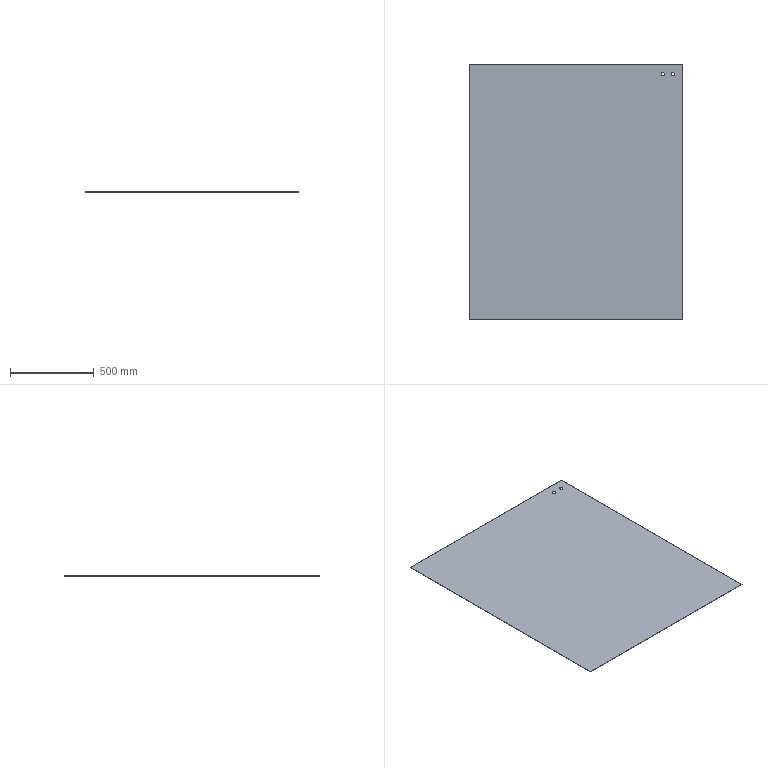Part | STEP file | ASND-0110-E63-HLTP01标准Lower机架-10 | 1 solid | 10 faces | box 1280 x 1530 x 2 mm | volume 3915543 mm3 | plane 6 | cylinder 4 | commonest cylinder face diameters 20 x4
STEP:
#1=CARTESIAN_POINT('',(0.,0.,0.));
#2=DIRECTION('',(0.,0.,1.));
#3=DIRECTION('',(1.,0.,0.));
#4=AXIS2_PLACEMENT_3D('',#1,#2,#3);
#5=CARTESIAN_POINT('',(-110.,-60.,0.));
#6=VERTEX_POINT('',#5);
#7=CARTESIAN_POINT('',(-110.,-60.,2.));
#8=VERTEX_POINT('',#7);
#9=CARTESIAN_POINT('',(-110.,-60.,-8.));
#10=DIRECTION('',(0.,0.,1.));
#11=VECTOR('',#10,1.);
#12=LINE('',#9,#11);
#13=CARTESIAN_POINT('',(-120.,-60.,-8.));
#14=DIRECTION('',(0.,0.,1.));
#15=DIRECTION('',(1.,0.,0.));
#16=AXIS2_PLACEMENT_3D('',#13,#14,#15);
#17=CYLINDRICAL_SURFACE('',#16,10.);
#18=CARTESIAN_POINT('',(6.283,0.));
#19=DIRECTION('',(0.,1.));
#20=VECTOR('',#19,1.);
#21=LINE('',#18,#20);
#22=(GEOMETRIC_REPRESENTATION_CONTEXT(2)PARAMETRIC_REPRESENTATION_CONTEXT()REPRESENTATION_CONTEXT('',''));
#23=DEFINITIONAL_REPRESENTATION('',(#21),#22);
#24=PCURVE('',#17,#23);
#25=CARTESIAN_POINT('',(-120.,-60.,-8.));
#26=DIRECTION('',(0.,0.,1.));
#27=DIRECTION('',(1.,0.,0.));
#28=AXIS2_PLACEMENT_3D('',#25,#26,#27);
#29=CYLINDRICAL_SURFACE('',#28,10.);
#30=CARTESIAN_POINT('',(0.,0.));
#31=DIRECTION('',(0.,1.));
#32=VECTOR('',#31,1.);
#33=LINE('',#30,#32);
#34=(GEOMETRIC_REPRESENTATION_CONTEXT(2)PARAMETRIC_REPRESENTATION_CONTEXT()REPRESENTATION_CONTEXT('',''));
#35=DEFINITIONAL_REPRESENTATION('',(#33),#34);
#36=PCURVE('',#29,#35);
#37=SURFACE_CURVE('',#12,(#24,#36),.PCURVE_S1.);
#38=EDGE_CURVE('',#6,#8,#37,.T.);
#39=ORIENTED_EDGE('',*,*,#38,.T.);
#40=CARTESIAN_POINT('',(-130.,-60.,2.));
#41=VERTEX_POINT('',#40);
#42=CARTESIAN_POINT('',(-120.,-60.,2.));
#43=DIRECTION('',(0.,0.,1.));
#44=DIRECTION('',(1.,0.,0.));
#45=AXIS2_PLACEMENT_3D('',#42,#43,#44);
#46=CIRCLE('',#45,10.);
#47=CARTESIAN_POINT('',(0.,10.));
#48=DIRECTION('',(1.,0.));
#49=VECTOR('',#48,1.);
#50=LINE('',#47,#49);
#51=(GEOMETRIC_REPRESENTATION_CONTEXT(2)PARAMETRIC_REPRESENTATION_CONTEXT()REPRESENTATION_CONTEXT('',''));
#52=DEFINITIONAL_REPRESENTATION('',(#50),#51);
#53=PCURVE('',#17,#52);
#54=CARTESIAN_POINT('',(0.,0.,2.));
#55=DIRECTION('',(0.,0.,1.));
#56=DIRECTION('',(0.7071,0.7071,0.));
#57=AXIS2_PLACEMENT_3D('',#54,#55,#56);
#58=PLANE('',#57);
#59=CARTESIAN_POINT('',(-127.279,42.426));
#60=DIRECTION('',(0.7071,-0.7071));
#61=AXIS2_PLACEMENT_2D('',#59,#60);
#62=CIRCLE('',#61,10.);
#63=(GEOMETRIC_REPRESENTATION_CONTEXT(2)PARAMETRIC_REPRESENTATION_CONTEXT()REPRESENTATION_CONTEXT('',''));
#64=DEFINITIONAL_REPRESENTATION('',(#62),#63);
#65=PCURVE('',#58,#64);
#66=SURFACE_CURVE('',#46,(#53,#65),.PCURVE_S1.);
#67=EDGE_CURVE('',#41,#8,#66,.T.);
#68=ORIENTED_EDGE('',*,*,#67,.F.);
#69=CARTESIAN_POINT('',(-130.,-60.,0.));
#70=VERTEX_POINT('',#69);
#71=CARTESIAN_POINT('',(-130.,-60.,-8.));
#72=DIRECTION('',(0.,0.,1.));
#73=VECTOR('',#72,1.);
#74=LINE('',#71,#73);
#75=CARTESIAN_POINT('',(3.142,0.));
#76=DIRECTION('',(0.,1.));
#77=VECTOR('',#76,1.);
#78=LINE('',#75,#77);
#79=(GEOMETRIC_REPRESENTATION_CONTEXT(2)PARAMETRIC_REPRESENTATION_CONTEXT()REPRESENTATION_CONTEXT('',''));
#80=DEFINITIONAL_REPRESENTATION('',(#78),#79);
#81=PCURVE('',#17,#80);
#82=CARTESIAN_POINT('',(3.142,0.));
#83=DIRECTION('',(0.,1.));
#84=VECTOR('',#83,1.);
#85=LINE('',#82,#84);
#86=(GEOMETRIC_REPRESENTATION_CONTEXT(2)PARAMETRIC_REPRESENTATION_CONTEXT()REPRESENTATION_CONTEXT('',''));
#87=DEFINITIONAL_REPRESENTATION('',(#85),#86);
#88=PCURVE('',#29,#87);
#89=SURFACE_CURVE('',#74,(#81,#88),.PCURVE_S1.);
#90=EDGE_CURVE('',#70,#41,#89,.T.);
#91=ORIENTED_EDGE('',*,*,#90,.F.);
#92=CARTESIAN_POINT('',(-120.,-60.,0.));
#93=DIRECTION('',(0.,0.,1.));
#94=DIRECTION('',(1.,0.,0.));
#95=AXIS2_PLACEMENT_3D('',#92,#93,#94);
#96=CIRCLE('',#95,10.);
#97=CARTESIAN_POINT('',(0.,8.));
#98=DIRECTION('',(1.,0.));
#99=VECTOR('',#98,1.);
#100=LINE('',#97,#99);
#101=(GEOMETRIC_REPRESENTATION_CONTEXT(2)PARAMETRIC_REPRESENTATION_CONTEXT()REPRESENTATION_CONTEXT('',''));
#102=DEFINITIONAL_REPRESENTATION('',(#100),#101);
#103=PCURVE('',#17,#102);
#104=CARTESIAN_POINT('',(0.,0.,0.));
#105=DIRECTION('',(0.,0.,1.));
#106=DIRECTION('',(0.7071,0.7071,0.));
#107=AXIS2_PLACEMENT_3D('',#104,#105,#106);
#108=PLANE('',#107);
#109=CARTESIAN_POINT('',(-127.279,42.426));
#110=DIRECTION('',(0.7071,-0.7071));
#111=AXIS2_PLACEMENT_2D('',#109,#110);
#112=CIRCLE('',#111,10.);
#113=(GEOMETRIC_REPRESENTATION_CONTEXT(2)PARAMETRIC_REPRESENTATION_CONTEXT()REPRESENTATION_CONTEXT('',''));
#114=DEFINITIONAL_REPRESENTATION('',(#112),#113);
#115=PCURVE('',#108,#114);
#116=SURFACE_CURVE('',#96,(#103,#115),.PCURVE_S1.);
#117=EDGE_CURVE('',#70,#6,#116,.T.);
#118=ORIENTED_EDGE('',*,*,#117,.T.);
#119=EDGE_LOOP('',(#39,#68,#91,#118));
#120=FACE_BOUND('',#119,.F.);
#121=ADVANCED_FACE('',(#120),#17,.F.);
#122=CARTESIAN_POINT('',(-170.,-60.,0.));
#123=VERTEX_POINT('',#122);
#124=CARTESIAN_POINT('',(-170.,-60.,2.));
#125=VERTEX_POINT('',#124);
#126=CARTESIAN_POINT('',(-170.,-60.,-8.));
#127=DIRECTION('',(0.,0.,1.));
#128=VECTOR('',#127,1.);
#129=LINE('',#126,#128);
#130=CARTESIAN_POINT('',(-180.,-60.,-8.));
#131=DIRECTION('',(0.,0.,1.));
#132=DIRECTION('',(1.,0.,0.));
#133=AXIS2_PLACEMENT_3D('',#130,#131,#132);
#134=CYLINDRICAL_SURFACE('',#133,10.);
#135=CARTESIAN_POINT('',(6.283,0.));
#136=DIRECTION('',(0.,1.));
#137=VECTOR('',#136,1.);
#138=LINE('',#135,#137);
#139=(GEOMETRIC_REPRESENTATION_CONTEXT(2)PARAMETRIC_REPRESENTATION_CONTEXT()REPRESENTATION_CONTEXT('',''));
#140=DEFINITIONAL_REPRESENTATION('',(#138),#139);
#141=PCURVE('',#134,#140);
#142=CARTESIAN_POINT('',(-180.,-60.,-8.));
#143=DIRECTION('',(0.,0.,1.));
#144=DIRECTION('',(1.,0.,0.));
#145=AXIS2_PLACEMENT_3D('',#142,#143,#144);
#146=CYLINDRICAL_SURFACE('',#145,10.);
#147=CARTESIAN_POINT('',(0.,0.));
#148=DIRECTION('',(0.,1.));
#149=VECTOR('',#148,1.);
#150=LINE('',#147,#149);
#151=(GEOMETRIC_REPRESENTATION_CONTEXT(2)PARAMETRIC_REPRESENTATION_CONTEXT()REPRESENTATION_CONTEXT('',''));
#152=DEFINITIONAL_REPRESENTATION('',(#150),#151);
#153=PCURVE('',#146,#152);
#154=SURFACE_CURVE('',#129,(#141,#153),.PCURVE_S1.);
#155=EDGE_CURVE('',#123,#125,#154,.T.);
#156=ORIENTED_EDGE('',*,*,#155,.T.);
#157=CARTESIAN_POINT('',(-190.,-60.,2.));
#158=VERTEX_POINT('',#157);
#159=CARTESIAN_POINT('',(-180.,-60.,2.));
#160=DIRECTION('',(0.,0.,1.));
#161=DIRECTION('',(1.,0.,0.));
#162=AXIS2_PLACEMENT_3D('',#159,#160,#161);
#163=CIRCLE('',#162,10.);
#164=CARTESIAN_POINT('',(0.,10.));
#165=DIRECTION('',(1.,0.));
#166=VECTOR('',#165,1.);
#167=LINE('',#164,#166);
#168=(GEOMETRIC_REPRESENTATION_CONTEXT(2)PARAMETRIC_REPRESENTATION_CONTEXT()REPRESENTATION_CONTEXT('',''));
#169=DEFINITIONAL_REPRESENTATION('',(#167),#168);
#170=PCURVE('',#134,#169);
#171=CARTESIAN_POINT('',(-169.706,84.853));
#172=DIRECTION('',(0.7071,-0.7071));
#173=AXIS2_PLACEMENT_2D('',#171,#172);
#174=CIRCLE('',#173,10.);
#175=(GEOMETRIC_REPRESENTATION_CONTEXT(2)PARAMETRIC_REPRESENTATION_CONTEXT()REPRESENTATION_CONTEXT('',''));
#176=DEFINITIONAL_REPRESENTATION('',(#174),#175);
#177=PCURVE('',#58,#176);
#178=SURFACE_CURVE('',#163,(#170,#177),.PCURVE_S1.);
#179=EDGE_CURVE('',#158,#125,#178,.T.);
#180=ORIENTED_EDGE('',*,*,#179,.F.);
#181=CARTESIAN_POINT('',(-190.,-60.,0.));
#182=VERTEX_POINT('',#181);
#183=CARTESIAN_POINT('',(-190.,-60.,-8.));
#184=DIRECTION('',(0.,0.,1.));
#185=VECTOR('',#184,1.);
#186=LINE('',#183,#185);
#187=CARTESIAN_POINT('',(3.142,0.));
#188=DIRECTION('',(0.,1.));
#189=VECTOR('',#188,1.);
#190=LINE('',#187,#189);
#191=(GEOMETRIC_REPRESENTATION_CONTEXT(2)PARAMETRIC_REPRESENTATION_CONTEXT()REPRESENTATION_CONTEXT('',''));
#192=DEFINITIONAL_REPRESENTATION('',(#190),#191);
#193=PCURVE('',#134,#192);
#194=CARTESIAN_POINT('',(3.142,0.));
#195=DIRECTION('',(0.,1.));
#196=VECTOR('',#195,1.);
#197=LINE('',#194,#196);
#198=(GEOMETRIC_REPRESENTATION_CONTEXT(2)PARAMETRIC_REPRESENTATION_CONTEXT()REPRESENTATION_CONTEXT('',''));
#199=DEFINITIONAL_REPRESENTATION('',(#197),#198);
#200=PCURVE('',#146,#199);
#201=SURFACE_CURVE('',#186,(#193,#200),.PCURVE_S1.);
#202=EDGE_CURVE('',#182,#158,#201,.T.);
#203=ORIENTED_EDGE('',*,*,#202,.F.);
#204=CARTESIAN_POINT('',(-180.,-60.,0.));
#205=DIRECTION('',(0.,0.,1.));
#206=DIRECTION('',(1.,0.,0.));
#207=AXIS2_PLACEMENT_3D('',#204,#205,#206);
#208=CIRCLE('',#207,10.);
#209=CARTESIAN_POINT('',(0.,8.));
#210=DIRECTION('',(1.,0.));
#211=VECTOR('',#210,1.);
#212=LINE('',#209,#211);
#213=(GEOMETRIC_REPRESENTATION_CONTEXT(2)PARAMETRIC_REPRESENTATION_CONTEXT()REPRESENTATION_CONTEXT('',''));
#214=DEFINITIONAL_REPRESENTATION('',(#212),#213);
#215=PCURVE('',#134,#214);
#216=CARTESIAN_POINT('',(-169.706,84.853));
#217=DIRECTION('',(0.7071,-0.7071));
#218=AXIS2_PLACEMENT_2D('',#216,#217);
#219=CIRCLE('',#218,10.);
#220=(GEOMETRIC_REPRESENTATION_CONTEXT(2)PARAMETRIC_REPRESENTATION_CONTEXT()REPRESENTATION_CONTEXT('',''));
#221=DEFINITIONAL_REPRESENTATION('',(#219),#220);
#222=PCURVE('',#108,#221);
#223=SURFACE_CURVE('',#208,(#215,#222),.PCURVE_S1.);
#224=EDGE_CURVE('',#182,#123,#223,.T.);
#225=ORIENTED_EDGE('',*,*,#224,.T.);
#226=EDGE_LOOP('',(#156,#180,#203,#225));
#227=FACE_BOUND('',#226,.F.);
#228=ADVANCED_FACE('',(#227),#134,.F.);
#229=CARTESIAN_POINT('',(-1340.,0.,0.));
#230=VERTEX_POINT('',#229);
#231=CARTESIAN_POINT('',(-1340.,-1530.,0.));
#232=VERTEX_POINT('',#231);
#233=CARTESIAN_POINT('',(-1340.,0.,0.));
#234=DIRECTION('',(0.,-1.,0.));
#235=VECTOR('',#234,1.);
#236=LINE('',#233,#235);
#237=CARTESIAN_POINT('',(-1340.,0.,2.));
#238=DIRECTION('',(1.,0.,0.));
#239=DIRECTION('',(0.,0.7071,0.7071));
#240=AXIS2_PLACEMENT_3D('',#237,#238,#239);
#241=PLANE('',#240);
#242=CARTESIAN_POINT('',(-1.414,-1.414));
#243=DIRECTION('',(-0.7071,0.7071));
#244=VECTOR('',#243,1.);
#245=LINE('',#242,#244);
#246=(GEOMETRIC_REPRESENTATION_CONTEXT(2)PARAMETRIC_REPRESENTATION_CONTEXT()REPRESENTATION_CONTEXT('',''));
#247=DEFINITIONAL_REPRESENTATION('',(#245),#246);
#248=PCURVE('',#241,#247);
#249=CARTESIAN_POINT('',(-947.523,947.523));
#250=DIRECTION('',(-0.7071,-0.7071));
#251=VECTOR('',#250,1.);
#252=LINE('',#249,#251);
#253=(GEOMETRIC_REPRESENTATION_CONTEXT(2)PARAMETRIC_REPRESENTATION_CONTEXT()REPRESENTATION_CONTEXT('',''));
#254=DEFINITIONAL_REPRESENTATION('',(#252),#253);
#255=PCURVE('',#108,#254);
#256=SURFACE_CURVE('',#236,(#248,#255),.PCURVE_S1.);
#257=EDGE_CURVE('',#230,#232,#256,.T.);
#258=ORIENTED_EDGE('',*,*,#257,.T.);
#259=CARTESIAN_POINT('',(-1340.,-1530.,2.));
#260=VERTEX_POINT('',#259);
#261=CARTESIAN_POINT('',(-1340.,-1530.,2.));
#262=DIRECTION('',(0.,0.,-1.));
#263=VECTOR('',#262,1.);
#264=LINE('',#261,#263);
#265=CARTESIAN_POINT('',(-1081.873,1081.873));
#266=DIRECTION('',(-0.7071,-0.7071));
#267=VECTOR('',#266,1.);
#268=LINE('',#265,#267);
#269=(GEOMETRIC_REPRESENTATION_CONTEXT(2)PARAMETRIC_REPRESENTATION_CONTEXT()REPRESENTATION_CONTEXT('',''));
#270=DEFINITIONAL_REPRESENTATION('',(#268),#269);
#271=PCURVE('',#241,#270);
#272=CARTESIAN_POINT('',(-1340.,-1530.,2.));
#273=DIRECTION('',(0.,1.,0.));
#274=DIRECTION('',(0.7071,0.,0.7071));
#275=AXIS2_PLACEMENT_3D('',#272,#273,#274);
#276=PLANE('',#275);
#277=CARTESIAN_POINT('',(0.,0.));
#278=DIRECTION('',(-0.7071,0.7071));
#279=VECTOR('',#278,1.);
#280=LINE('',#277,#279);
#281=(GEOMETRIC_REPRESENTATION_CONTEXT(2)PARAMETRIC_REPRESENTATION_CONTEXT()REPRESENTATION_CONTEXT('',''));
#282=DEFINITIONAL_REPRESENTATION('',(#280),#281);
#283=PCURVE('',#276,#282);
#284=SURFACE_CURVE('',#264,(#271,#283),.PCURVE_S1.);
#285=EDGE_CURVE('',#260,#232,#284,.T.);
#286=ORIENTED_EDGE('',*,*,#285,.F.);
#287=CARTESIAN_POINT('',(-1340.,0.,2.));
#288=VERTEX_POINT('',#287);
#289=CARTESIAN_POINT('',(-1340.,0.,2.));
#290=DIRECTION('',(0.,-1.,0.));
#291=VECTOR('',#290,1.);
#292=LINE('',#289,#291);
#293=CARTESIAN_POINT('',(0.,0.));
#294=DIRECTION('',(-0.7071,0.7071));
#295=VECTOR('',#294,1.);
#296=LINE('',#293,#295);
#297=(GEOMETRIC_REPRESENTATION_CONTEXT(2)PARAMETRIC_REPRESENTATION_CONTEXT()REPRESENTATION_CONTEXT('',''));
#298=DEFINITIONAL_REPRESENTATION('',(#296),#297);
#299=PCURVE('',#241,#298);
#300=CARTESIAN_POINT('',(-947.523,947.523));
#301=DIRECTION('',(-0.7071,-0.7071));
#302=VECTOR('',#301,1.);
#303=LINE('',#300,#302);
#304=(GEOMETRIC_REPRESENTATION_CONTEXT(2)PARAMETRIC_REPRESENTATION_CONTEXT()REPRESENTATION_CONTEXT('',''));
#305=DEFINITIONAL_REPRESENTATION('',(#303),#304);
#306=PCURVE('',#58,#305);
#307=SURFACE_CURVE('',#292,(#299,#306),.PCURVE_S1.);
#308=EDGE_CURVE('',#288,#260,#307,.T.);
#309=ORIENTED_EDGE('',*,*,#308,.F.);
#310=CARTESIAN_POINT('',(-1340.,0.,2.));
#311=DIRECTION('',(0.,0.,-1.));
#312=VECTOR('',#311,1.);
#313=LINE('',#310,#312);
#314=CARTESIAN_POINT('',(0.,0.));
#315=DIRECTION('',(-0.7071,-0.7071));
#316=VECTOR('',#315,1.);
#317=LINE('',#314,#316);
#318=(GEOMETRIC_REPRESENTATION_CONTEXT(2)PARAMETRIC_REPRESENTATION_CONTEXT()REPRESENTATION_CONTEXT('',''));
#319=DEFINITIONAL_REPRESENTATION('',(#317),#318);
#320=PCURVE('',#241,#319);
#321=CARTESIAN_POINT('',(-1340.,0.,2.));
#322=DIRECTION('',(0.,-1.,0.));
#323=DIRECTION('',(0.7071,0.,0.7071));
#324=AXIS2_PLACEMENT_3D('',#321,#322,#323);
#325=PLANE('',#324);
#326=CARTESIAN_POINT('',(0.,0.));
#327=DIRECTION('',(-0.7071,-0.7071));
#328=VECTOR('',#327,1.);
#329=LINE('',#326,#328);
#330=(GEOMETRIC_REPRESENTATION_CONTEXT(2)PARAMETRIC_REPRESENTATION_CONTEXT()REPRESENTATION_CONTEXT('',''));
#331=DEFINITIONAL_REPRESENTATION('',(#329),#330);
#332=PCURVE('',#325,#331);
#333=SURFACE_CURVE('',#313,(#320,#332),.PCURVE_S1.);
#334=EDGE_CURVE('',#288,#230,#333,.T.);
#335=ORIENTED_EDGE('',*,*,#334,.T.);
#336=EDGE_LOOP('',(#258,#286,#309,#335));
#337=FACE_BOUND('',#336,.T.);
#338=ADVANCED_FACE('',(#337),#241,.F.);
#339=CARTESIAN_POINT('',(-60.,-1530.,0.));
#340=VERTEX_POINT('',#339);
#341=CARTESIAN_POINT('',(-1340.,-1530.,0.));
#342=DIRECTION('',(1.,0.,0.));
#343=VECTOR('',#342,1.);
#344=LINE('',#341,#343);
#345=CARTESIAN_POINT('',(-1.414,1.414));
#346=DIRECTION('',(0.7071,0.7071));
#347=VECTOR('',#346,1.);
#348=LINE('',#345,#347);
#349=(GEOMETRIC_REPRESENTATION_CONTEXT(2)PARAMETRIC_REPRESENTATION_CONTEXT()REPRESENTATION_CONTEXT('',''));
#350=DEFINITIONAL_REPRESENTATION('',(#348),#349);
#351=PCURVE('',#276,#350);
#352=CARTESIAN_POINT('',(-2029.396,-134.35));
#353=DIRECTION('',(0.7071,-0.7071));
#354=VECTOR('',#353,1.);
#355=LINE('',#352,#354);
#356=(GEOMETRIC_REPRESENTATION_CONTEXT(2)PARAMETRIC_REPRESENTATION_CONTEXT()REPRESENTATION_CONTEXT('',''));
#357=DEFINITIONAL_REPRESENTATION('',(#355),#356);
#358=PCURVE('',#108,#357);
#359=SURFACE_CURVE('',#344,(#351,#358),.PCURVE_S1.);
#360=EDGE_CURVE('',#232,#340,#359,.T.);
#361=ORIENTED_EDGE('',*,*,#360,.T.);
#362=CARTESIAN_POINT('',(-60.,-1530.,2.));
#363=VERTEX_POINT('',#362);
#364=CARTESIAN_POINT('',(-60.,-1530.,2.));
#365=DIRECTION('',(0.,0.,-1.));
#366=VECTOR('',#365,1.);
#367=LINE('',#364,#366);
#368=CARTESIAN_POINT('',(905.097,905.097));
#369=DIRECTION('',(-0.7071,0.7071));
#370=VECTOR('',#369,1.);
#371=LINE('',#368,#370);
#372=(GEOMETRIC_REPRESENTATION_CONTEXT(2)PARAMETRIC_REPRESENTATION_CONTEXT()REPRESENTATION_CONTEXT('',''));
#373=DEFINITIONAL_REPRESENTATION('',(#371),#372);
#374=PCURVE('',#276,#373);
#375=CARTESIAN_POINT('',(-60.,0.,2.));
#376=DIRECTION('',(-1.,0.,0.));
#377=DIRECTION('',(0.,0.7071,0.7071));
#378=AXIS2_PLACEMENT_3D('',#375,#376,#377);
#379=PLANE('',#378);
#380=CARTESIAN_POINT('',(-1081.873,-1081.873));
#381=DIRECTION('',(-0.7071,0.7071));
#382=VECTOR('',#381,1.);
#383=LINE('',#380,#382);
#384=(GEOMETRIC_REPRESENTATION_CONTEXT(2)PARAMETRIC_REPRESENTATION_CONTEXT()REPRESENTATION_CONTEXT('',''));
#385=DEFINITIONAL_REPRESENTATION('',(#383),#384);
#386=PCURVE('',#379,#385);
#387=SURFACE_CURVE('',#367,(#374,#386),.PCURVE_S1.);
#388=EDGE_CURVE('',#363,#340,#387,.T.);
#389=ORIENTED_EDGE('',*,*,#388,.F.);
#390=CARTESIAN_POINT('',(-1340.,-1530.,2.));
#391=DIRECTION('',(1.,0.,0.));
#392=VECTOR('',#391,1.);
#393=LINE('',#390,#392);
#394=CARTESIAN_POINT('',(0.,0.));
#395=DIRECTION('',(0.7071,0.7071));
#396=VECTOR('',#395,1.);
#397=LINE('',#394,#396);
#398=(GEOMETRIC_REPRESENTATION_CONTEXT(2)PARAMETRIC_REPRESENTATION_CONTEXT()REPRESENTATION_CONTEXT('',''));
#399=DEFINITIONAL_REPRESENTATION('',(#397),#398);
#400=PCURVE('',#276,#399);
#401=CARTESIAN_POINT('',(-2029.396,-134.35));
#402=DIRECTION('',(0.7071,-0.7071));
#403=VECTOR('',#402,1.);
#404=LINE('',#401,#403);
#405=(GEOMETRIC_REPRESENTATION_CONTEXT(2)PARAMETRIC_REPRESENTATION_CONTEXT()REPRESENTATION_CONTEXT('',''));
#406=DEFINITIONAL_REPRESENTATION('',(#404),#405);
#407=PCURVE('',#58,#406);
#408=SURFACE_CURVE('',#393,(#400,#407),.PCURVE_S1.);
#409=EDGE_CURVE('',#260,#363,#408,.T.);
#410=ORIENTED_EDGE('',*,*,#409,.F.);
#411=ORIENTED_EDGE('',*,*,#285,.T.);
#412=EDGE_LOOP('',(#361,#389,#410,#411));
#413=FACE_BOUND('',#412,.T.);
#414=ADVANCED_FACE('',(#413),#276,.F.);
#415=CARTESIAN_POINT('',(-60.,0.,0.));
#416=VERTEX_POINT('',#415);
#417=CARTESIAN_POINT('',(-60.,-1530.,0.));
#418=DIRECTION('',(0.,1.,0.));
#419=VECTOR('',#418,1.);
#420=LINE('',#417,#419);
#421=CARTESIAN_POINT('',(-1083.288,-1080.459));
#422=DIRECTION('',(0.7071,0.7071));
#423=VECTOR('',#422,1.);
#424=LINE('',#421,#423);
#425=(GEOMETRIC_REPRESENTATION_CONTEXT(2)PARAMETRIC_REPRESENTATION_CONTEXT()REPRESENTATION_CONTEXT('',''));
#426=DEFINITIONAL_REPRESENTATION('',(#424),#425);
#427=PCURVE('',#379,#426);
#428=CARTESIAN_POINT('',(-1124.3,-1039.447));
#429=DIRECTION('',(0.7071,0.7071));
#430=VECTOR('',#429,1.);
#431=LINE('',#428,#430);
#432=(GEOMETRIC_REPRESENTATION_CONTEXT(2)PARAMETRIC_REPRESENTATION_CONTEXT()REPRESENTATION_CONTEXT('',''));
#433=DEFINITIONAL_REPRESENTATION('',(#431),#432);
#434=PCURVE('',#108,#433);
#435=SURFACE_CURVE('',#420,(#427,#434),.PCURVE_S1.);
#436=EDGE_CURVE('',#340,#416,#435,.T.);
#437=ORIENTED_EDGE('',*,*,#436,.T.);
#438=CARTESIAN_POINT('',(-60.,0.,2.));
#439=VERTEX_POINT('',#438);
#440=CARTESIAN_POINT('',(-60.,0.,2.));
#441=DIRECTION('',(0.,0.,-1.));
#442=VECTOR('',#441,1.);
#443=LINE('',#440,#442);
#444=CARTESIAN_POINT('',(0.,0.));
#445=DIRECTION('',(-0.7071,0.7071));
#446=VECTOR('',#445,1.);
#447=LINE('',#444,#446);
#448=(GEOMETRIC_REPRESENTATION_CONTEXT(2)PARAMETRIC_REPRESENTATION_CONTEXT()REPRESENTATION_CONTEXT('',''));
#449=DEFINITIONAL_REPRESENTATION('',(#447),#448);
#450=PCURVE('',#379,#449);
#451=CARTESIAN_POINT('',(905.097,-905.097));
#452=DIRECTION('',(-0.7071,-0.7071));
#453=VECTOR('',#452,1.);
#454=LINE('',#451,#453);
#455=(GEOMETRIC_REPRESENTATION_CONTEXT(2)PARAMETRIC_REPRESENTATION_CONTEXT()REPRESENTATION_CONTEXT('',''));
#456=DEFINITIONAL_REPRESENTATION('',(#454),#455);
#457=PCURVE('',#325,#456);
#458=SURFACE_CURVE('',#443,(#450,#457),.PCURVE_S1.);
#459=EDGE_CURVE('',#439,#416,#458,.T.);
#460=ORIENTED_EDGE('',*,*,#459,.F.);
#461=CARTESIAN_POINT('',(-60.,-1530.,2.));
#462=DIRECTION('',(0.,1.,0.));
#463=VECTOR('',#462,1.);
#464=LINE('',#461,#463);
#465=CARTESIAN_POINT('',(-1081.873,-1081.873));
#466=DIRECTION('',(0.7071,0.7071));
#467=VECTOR('',#466,1.);
#468=LINE('',#465,#467);
#469=(GEOMETRIC_REPRESENTATION_CONTEXT(2)PARAMETRIC_REPRESENTATION_CONTEXT()REPRESENTATION_CONTEXT('',''));
#470=DEFINITIONAL_REPRESENTATION('',(#468),#469);
#471=PCURVE('',#379,#470);
#472=CARTESIAN_POINT('',(-1124.3,-1039.447));
#473=DIRECTION('',(0.7071,0.7071));
#474=VECTOR('',#473,1.);
#475=LINE('',#472,#474);
#476=(GEOMETRIC_REPRESENTATION_CONTEXT(2)PARAMETRIC_REPRESENTATION_CONTEXT()REPRESENTATION_CONTEXT('',''));
#477=DEFINITIONAL_REPRESENTATION('',(#475),#476);
#478=PCURVE('',#58,#477);
#479=SURFACE_CURVE('',#464,(#471,#478),.PCURVE_S1.);
#480=EDGE_CURVE('',#363,#439,#479,.T.);
#481=ORIENTED_EDGE('',*,*,#480,.F.);
#482=ORIENTED_EDGE('',*,*,#388,.T.);
#483=EDGE_LOOP('',(#437,#460,#481,#482));
#484=FACE_BOUND('',#483,.T.);
#485=ADVANCED_FACE('',(#484),#379,.F.);
#486=CARTESIAN_POINT('',(-60.,0.,0.));
#487=DIRECTION('',(-1.,0.,0.));
#488=VECTOR('',#487,1.);
#489=LINE('',#486,#488);
#490=CARTESIAN_POINT('',(903.682,-906.511));
#491=DIRECTION('',(-0.7071,0.7071));
#492=VECTOR('',#491,1.);
#493=LINE('',#490,#492);
#494=(GEOMETRIC_REPRESENTATION_CONTEXT(2)PARAMETRIC_REPRESENTATION_CONTEXT()REPRESENTATION_CONTEXT('',''));
#495=DEFINITIONAL_REPRESENTATION('',(#493),#494);
#496=PCURVE('',#325,#495);
#497=CARTESIAN_POINT('',(-42.426,42.426));
#498=DIRECTION('',(-0.7071,0.7071));
#499=VECTOR('',#498,1.);
#500=LINE('',#497,#499);
#501=(GEOMETRIC_REPRESENTATION_CONTEXT(2)PARAMETRIC_REPRESENTATION_CONTEXT()REPRESENTATION_CONTEXT('',''));
#502=DEFINITIONAL_REPRESENTATION('',(#500),#501);
#503=PCURVE('',#108,#502);
#504=SURFACE_CURVE('',#489,(#496,#503),.PCURVE_S1.);
#505=EDGE_CURVE('',#416,#230,#504,.T.);
#506=ORIENTED_EDGE('',*,*,#505,.T.);
#507=ORIENTED_EDGE('',*,*,#334,.F.);
#508=CARTESIAN_POINT('',(-60.,0.,2.));
#509=DIRECTION('',(-1.,0.,0.));
#510=VECTOR('',#509,1.);
#511=LINE('',#508,#510);
#512=CARTESIAN_POINT('',(905.097,-905.097));
#513=DIRECTION('',(-0.7071,0.7071));
#514=VECTOR('',#513,1.);
#515=LINE('',#512,#514);
#516=(GEOMETRIC_REPRESENTATION_CONTEXT(2)PARAMETRIC_REPRESENTATION_CONTEXT()REPRESENTATION_CONTEXT('',''));
#517=DEFINITIONAL_REPRESENTATION('',(#515),#516);
#518=PCURVE('',#325,#517);
#519=CARTESIAN_POINT('',(-42.426,42.426));
#520=DIRECTION('',(-0.7071,0.7071));
#521=VECTOR('',#520,1.);
#522=LINE('',#519,#521);
#523=(GEOMETRIC_REPRESENTATION_CONTEXT(2)PARAMETRIC_REPRESENTATION_CONTEXT()REPRESENTATION_CONTEXT('',''));
#524=DEFINITIONAL_REPRESENTATION('',(#522),#523);
#525=PCURVE('',#58,#524);
#526=SURFACE_CURVE('',#511,(#518,#525),.PCURVE_S1.);
#527=EDGE_CURVE('',#439,#288,#526,.T.);
#528=ORIENTED_EDGE('',*,*,#527,.F.);
#529=ORIENTED_EDGE('',*,*,#459,.T.);
#530=EDGE_LOOP('',(#506,#507,#528,#529));
#531=FACE_BOUND('',#530,.T.);
#532=ADVANCED_FACE('',(#531),#325,.F.);
#533=ORIENTED_EDGE('',*,*,#308,.T.);
#534=ORIENTED_EDGE('',*,*,#409,.T.);
#535=ORIENTED_EDGE('',*,*,#480,.T.);
#536=ORIENTED_EDGE('',*,*,#527,.T.);
#537=EDGE_LOOP('',(#533,#534,#535,#536));
#538=FACE_BOUND('',#537,.T.);
#539=CARTESIAN_POINT('',(-120.,-60.,2.));
#540=DIRECTION('',(0.,0.,1.));
#541=DIRECTION('',(1.,0.,0.));
#542=AXIS2_PLACEMENT_3D('',#539,#540,#541);
#543=CIRCLE('',#542,10.);
#544=CARTESIAN_POINT('',(-127.279,42.426));
#545=DIRECTION('',(0.7071,-0.7071));
#546=AXIS2_PLACEMENT_2D('',#544,#545);
#547=CIRCLE('',#546,10.);
#548=(GEOMETRIC_REPRESENTATION_CONTEXT(2)PARAMETRIC_REPRESENTATION_CONTEXT()REPRESENTATION_CONTEXT('',''));
#549=DEFINITIONAL_REPRESENTATION('',(#547),#548);
#550=PCURVE('',#58,#549);
#551=CARTESIAN_POINT('',(0.,10.));
#552=DIRECTION('',(1.,0.));
#553=VECTOR('',#552,1.);
#554=LINE('',#551,#553);
#555=(GEOMETRIC_REPRESENTATION_CONTEXT(2)PARAMETRIC_REPRESENTATION_CONTEXT()REPRESENTATION_CONTEXT('',''));
#556=DEFINITIONAL_REPRESENTATION('',(#554),#555);
#557=PCURVE('',#29,#556);
#558=SURFACE_CURVE('',#543,(#550,#557),.PCURVE_S1.);
#559=EDGE_CURVE('',#8,#41,#558,.T.);
#560=ORIENTED_EDGE('',*,*,#559,.F.);
#561=ORIENTED_EDGE('',*,*,#67,.F.);
#562=EDGE_LOOP('',(#560,#561));
#563=FACE_BOUND('',#562,.T.);
#564=CARTESIAN_POINT('',(-180.,-60.,2.));
#565=DIRECTION('',(0.,0.,1.));
#566=DIRECTION('',(1.,0.,0.));
#567=AXIS2_PLACEMENT_3D('',#564,#565,#566);
#568=CIRCLE('',#567,10.);
#569=CARTESIAN_POINT('',(-169.706,84.853));
#570=DIRECTION('',(0.7071,-0.7071));
#571=AXIS2_PLACEMENT_2D('',#569,#570);
#572=CIRCLE('',#571,10.);
#573=(GEOMETRIC_REPRESENTATION_CONTEXT(2)PARAMETRIC_REPRESENTATION_CONTEXT()REPRESENTATION_CONTEXT('',''));
#574=DEFINITIONAL_REPRESENTATION('',(#572),#573);
#575=PCURVE('',#58,#574);
#576=CARTESIAN_POINT('',(0.,10.));
#577=DIRECTION('',(1.,0.));
#578=VECTOR('',#577,1.);
#579=LINE('',#576,#578);
#580=(GEOMETRIC_REPRESENTATION_CONTEXT(2)PARAMETRIC_REPRESENTATION_CONTEXT()REPRESENTATION_CONTEXT('',''));
#581=DEFINITIONAL_REPRESENTATION('',(#579),#580);
#582=PCURVE('',#146,#581);
#583=SURFACE_CURVE('',#568,(#575,#582),.PCURVE_S1.);
#584=EDGE_CURVE('',#125,#158,#583,.T.);
#585=ORIENTED_EDGE('',*,*,#584,.F.);
#586=ORIENTED_EDGE('',*,*,#179,.F.);
#587=EDGE_LOOP('',(#585,#586));
#588=FACE_BOUND('',#587,.T.);
#589=ADVANCED_FACE('',(#538,#563,#588),#58,.T.);
#590=ORIENTED_EDGE('',*,*,#257,.F.);
#591=ORIENTED_EDGE('',*,*,#505,.F.);
#592=ORIENTED_EDGE('',*,*,#436,.F.);
#593=ORIENTED_EDGE('',*,*,#360,.F.);
#594=EDGE_LOOP('',(#590,#591,#592,#593));
#595=FACE_BOUND('',#594,.T.);
#596=CARTESIAN_POINT('',(-120.,-60.,0.));
#597=DIRECTION('',(0.,0.,1.));
#598=DIRECTION('',(1.,0.,0.));
#599=AXIS2_PLACEMENT_3D('',#596,#597,#598);
#600=CIRCLE('',#599,10.);
#601=CARTESIAN_POINT('',(-127.279,42.426));
#602=DIRECTION('',(0.7071,-0.7071));
#603=AXIS2_PLACEMENT_2D('',#601,#602);
#604=CIRCLE('',#603,10.);
#605=(GEOMETRIC_REPRESENTATION_CONTEXT(2)PARAMETRIC_REPRESENTATION_CONTEXT()REPRESENTATION_CONTEXT('',''));
#606=DEFINITIONAL_REPRESENTATION('',(#604),#605);
#607=PCURVE('',#108,#606);
#608=CARTESIAN_POINT('',(0.,8.));
#609=DIRECTION('',(1.,0.));
#610=VECTOR('',#609,1.);
#611=LINE('',#608,#610);
#612=(GEOMETRIC_REPRESENTATION_CONTEXT(2)PARAMETRIC_REPRESENTATION_CONTEXT()REPRESENTATION_CONTEXT('',''));
#613=DEFINITIONAL_REPRESENTATION('',(#611),#612);
#614=PCURVE('',#29,#613);
#615=SURFACE_CURVE('',#600,(#607,#614),.PCURVE_S1.);
#616=EDGE_CURVE('',#6,#70,#615,.T.);
#617=ORIENTED_EDGE('',*,*,#616,.T.);
#618=ORIENTED_EDGE('',*,*,#117,.T.);
#619=EDGE_LOOP('',(#617,#618));
#620=FACE_BOUND('',#619,.T.);
#621=CARTESIAN_POINT('',(-180.,-60.,0.));
#622=DIRECTION('',(0.,0.,1.));
#623=DIRECTION('',(1.,0.,0.));
#624=AXIS2_PLACEMENT_3D('',#621,#622,#623);
#625=CIRCLE('',#624,10.);
#626=CARTESIAN_POINT('',(-169.706,84.853));
#627=DIRECTION('',(0.7071,-0.7071));
#628=AXIS2_PLACEMENT_2D('',#626,#627);
#629=CIRCLE('',#628,10.);
#630=(GEOMETRIC_REPRESENTATION_CONTEXT(2)PARAMETRIC_REPRESENTATION_CONTEXT()REPRESENTATION_CONTEXT('',''));
#631=DEFINITIONAL_REPRESENTATION('',(#629),#630);
#632=PCURVE('',#108,#631);
#633=CARTESIAN_POINT('',(0.,8.));
#634=DIRECTION('',(1.,0.));
#635=VECTOR('',#634,1.);
#636=LINE('',#633,#635);
#637=(GEOMETRIC_REPRESENTATION_CONTEXT(2)PARAMETRIC_REPRESENTATION_CONTEXT()REPRESENTATION_CONTEXT('',''));
#638=DEFINITIONAL_REPRESENTATION('',(#636),#637);
#639=PCURVE('',#146,#638);
#640=SURFACE_CURVE('',#625,(#632,#639),.PCURVE_S1.);
#641=EDGE_CURVE('',#123,#182,#640,.T.);
#642=ORIENTED_EDGE('',*,*,#641,.T.);
#643=ORIENTED_EDGE('',*,*,#224,.T.);
#644=EDGE_LOOP('',(#642,#643));
#645=FACE_BOUND('',#644,.T.);
#646=ADVANCED_FACE('',(#595,#620,#645),#108,.F.);
#647=ORIENTED_EDGE('',*,*,#584,.F.);
#648=ORIENTED_EDGE('',*,*,#155,.F.);
#649=ORIENTED_EDGE('',*,*,#641,.T.);
#650=ORIENTED_EDGE('',*,*,#202,.T.);
#651=EDGE_LOOP('',(#647,#648,#649,#650));
#652=FACE_BOUND('',#651,.F.);
#653=ADVANCED_FACE('',(#652),#146,.F.);
#654=ORIENTED_EDGE('',*,*,#559,.F.);
#655=ORIENTED_EDGE('',*,*,#38,.F.);
#656=ORIENTED_EDGE('',*,*,#616,.T.);
#657=ORIENTED_EDGE('',*,*,#90,.T.);
#658=EDGE_LOOP('',(#654,#655,#656,#657));
#659=FACE_BOUND('',#658,.F.);
#660=ADVANCED_FACE('',(#659),#29,.F.);
#661=CLOSED_SHELL('',(#121,#228,#338,#414,#485,#532,#589,#646,#653,#660));
#662=MANIFOLD_SOLID_BREP('',#661);
#663=(LENGTH_UNIT()NAMED_UNIT(*)SI_UNIT(.MILLI.,.METRE.));
#664=UNCERTAINTY_MEASURE_WITH_UNIT(LENGTH_MEASURE(0.0000001),#663,'','');
#665=(NAMED_UNIT(*)PLANE_ANGLE_UNIT()SI_UNIT($,.RADIAN.));
#666=(NAMED_UNIT(*)SI_UNIT($,.STERADIAN.)SOLID_ANGLE_UNIT());
#667=(GEOMETRIC_REPRESENTATION_CONTEXT(3)GLOBAL_UNCERTAINTY_ASSIGNED_CONTEXT((#664))GLOBAL_UNIT_ASSIGNED_CONTEXT((#663,#665,#666))REPRESENTATION_CONTEXT('',''));
#668=ADVANCED_BREP_SHAPE_REPRESENTATION('',(#4,#662),#667);